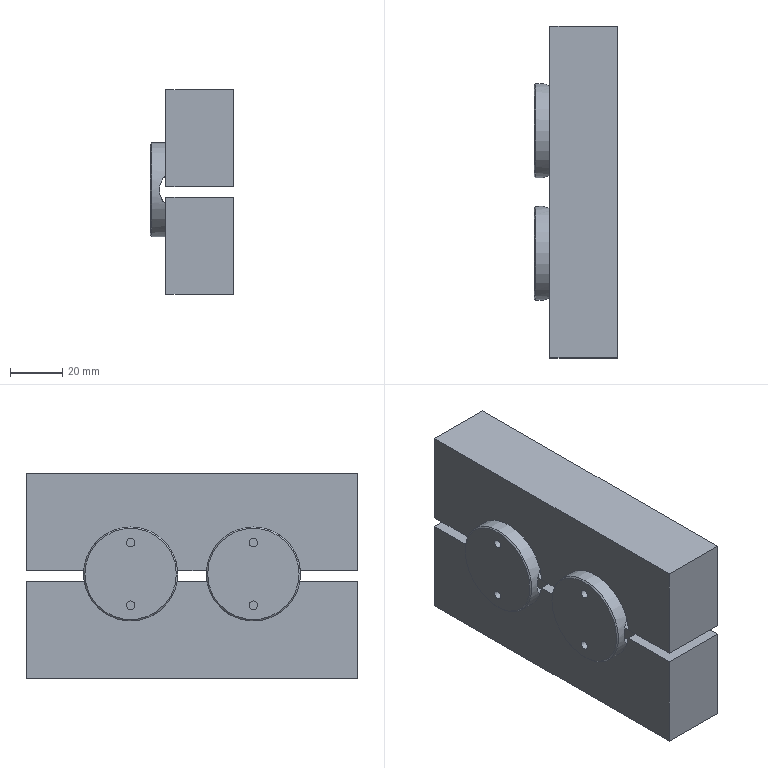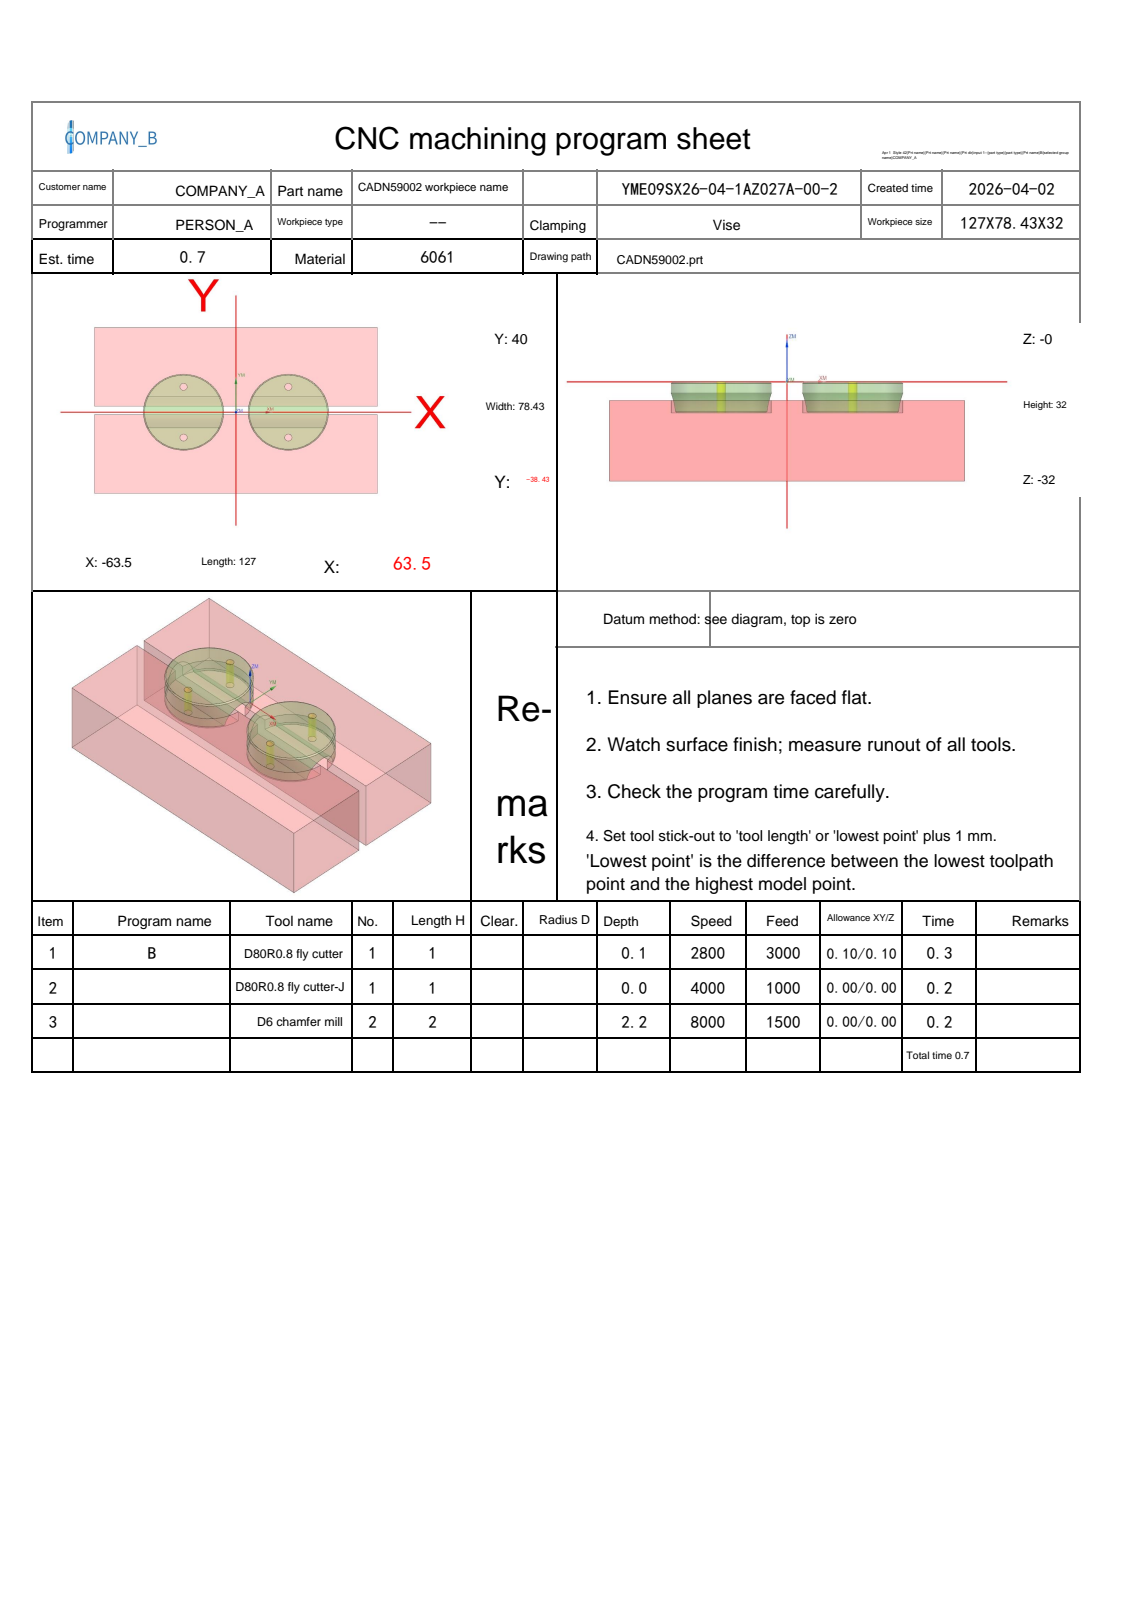NC program | NX | posted by the shop | part box 32 x 127 x 78.432 mm
Whole program:
%
O0001
(Machine time: 1.32 MIN)
(===Total Tool:2===)
(T1=D80R0.8 fly cutter D=80.  R=0.8  D-  H01 Z=-0.   )
(T2=D6 chamfer mill   D=6.   R=0.   D-  H02 Z=-2.2  )
G80 G90 G17 G49 G40
G91 G28 Z0
M01
N1 T01 M06
(D80R0.8 fly cutter  D=80. R=0.8 H=01 ce=0.10 di=0.10)
G00 G90 G54 X93.522 Y3.248 M03 S2800
G43 H01 Z20.
M08
Z3.525
G01 Z1.525 F3000.
X81.528 Y2.831
X-81.528 Y-2.831
X-93.522 Y-3.248
Z3.525
G00 X93.522 Y3.248
Z3.05
G01 Z1.05
X81.528 Y2.831
X-81.528 Y-2.831
X-93.522 Y-3.248
Z3.05
G00 X93.522 Y3.248
Z2.575
G01 Z.575
X81.528 Y2.831
X-81.528 Y-2.831
X-93.522 Y-3.248
Z2.575
G00 X93.522 Y3.248
Z2.1
G01 Z.1
X81.528 Y2.831
X-81.528 Y-2.831
X-93.522 Y-3.248
Z2.1
G00 Z20.
G91 G28 Z0.0
M05
M09
G91 G28 Z0.0
M01
N2 T01 M06
(D80R0.8 fly cutter-J  D=80. R=0.8 H=01 ce=0.00 di=0.00)
G00 G90 G54 X93.424 Y3.24 M03 S4000
G43 H01 Z20.
M08
Z2.
G01 Z0.0 F1000.
X81.43 Y2.824
X-81.43 Y-2.824
X-93.424 Y-3.24
Z2.
G00 Z20.
G91 G28 Z0.0
M05
M09
G91 G28 Z0.0
M01
N3 T02 M06
(D6 chamfer mill  D=6. R=0. H=02 ce=0.00 di=0.00)
G00 G90 G54 X-23.5 Y12. M03 S8000
G43 H02 Z20.
M08
G98 G81 X-23.5 Y12. Z-2.2 R3. F1000.
Y-12.
X23.5 Y12.
Y-12.
G80
G00 Z20.
G00 G90 X-24.699 Y19.864 M03 S6500
Z20.
Z.3
G01 Z-1.2 F1500.
G03 X-23.5 Y18.7 I1.199 J.036
G02 X-4.8 Y0.0 I0.0 J-18.7
X-23.5 Y-18.7 I-18.7 J0.0
X-42.2 Y0.0 I0.0 J18.7
X-41.017 Y6.544 I18.7 J0.0
G01 X-40.947 Y6.73
G02 X-30.23 Y17.447 I17.447 J-6.73
X-28.545 Y18.007 I6.73 J-17.447
X-26.82 Y18.403 I5.045 J-18.007
X-25.812 Y18.556 I3.32 J-18.403
X-23.5 Y18.7 I2.312 J-18.556
X-23.1 Y18.696 I0.0 J-18.7
G01 X-23.074 Y18.695
G03 X-21.876 Y19.834 I0.0 J1.2
G01 Z.3
G00 Z20.
X22.301 Y19.864
Z.3
G01 Z-1.2
G03 X23.5 Y18.7 I1.199 J.036
G02 X23.759 Y18.698 I0.0 J-18.7
X42.2 Y0.0 I-.259 J-18.698
X23.5 Y-18.7 I-18.7 J0.0
X4.8 Y0.0 I0.0 J18.7
X22.817 Y18.688 I18.7 J0.0
X23.5 Y18.7 I.683 J-18.688
X23.759 Y18.698 I0.0 J-18.7
G01 X23.9 Y18.696
X23.926 Y18.695
G03 X25.124 Y19.834 I0.0 J1.2
G01 Z.3
G00 Z20.
M05
M09
G91 G28 Z0.0
G91 G28 Y0.0
M30
%